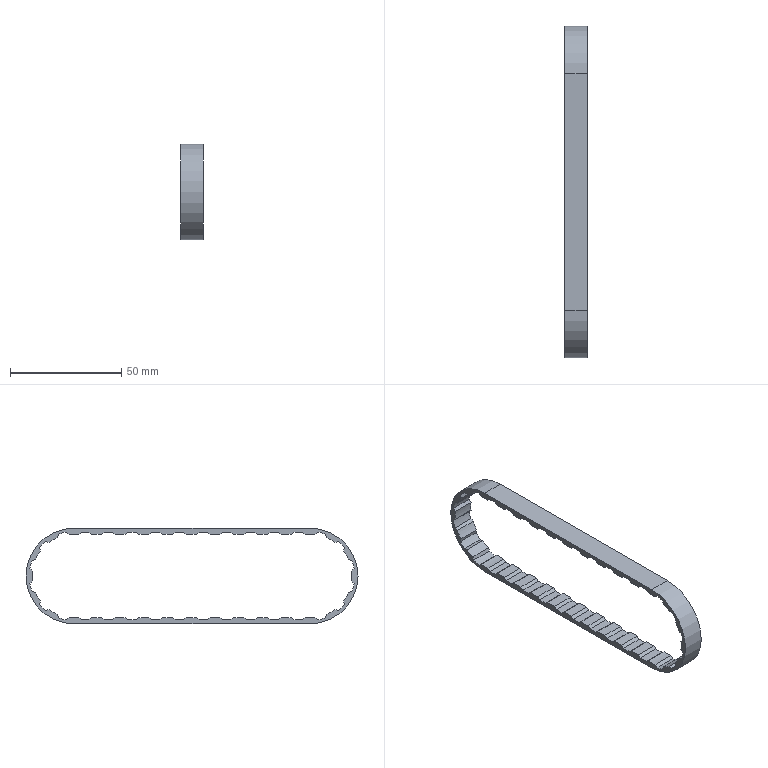Part | NX | features CPROJ 5, DATUM_CSYS 4, EXTRUDE 3, SKETCH 3, EXTRACT_BODY 2, TRIM BODY 2, Container 1, Delete Body 1, Geometry Instance 1, Pattern Geometry 1, UNITE 1 | 1 solid | 134 faces | box 10 x 149 x 43 mm | volume 7788 mm3 | plane 106 | cylinder 28 | commonest cylinder face diameters 37.525 x14 40 x12 43 x2